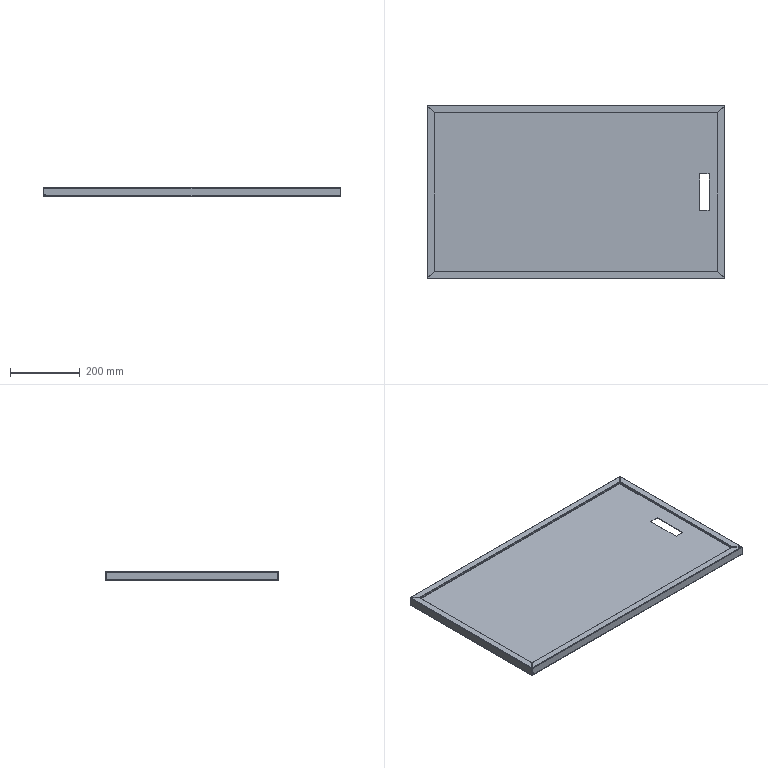Part | SolidWorks | features MirrorStock 1 | 1 solid | 78 faces | box 851 x 496 x 26.5 mm | volume 797153 mm3 | plane 42 | cylinder 20 | spline 16 | commonest cylinder face diameters 1 x8 4 x8 5 x4